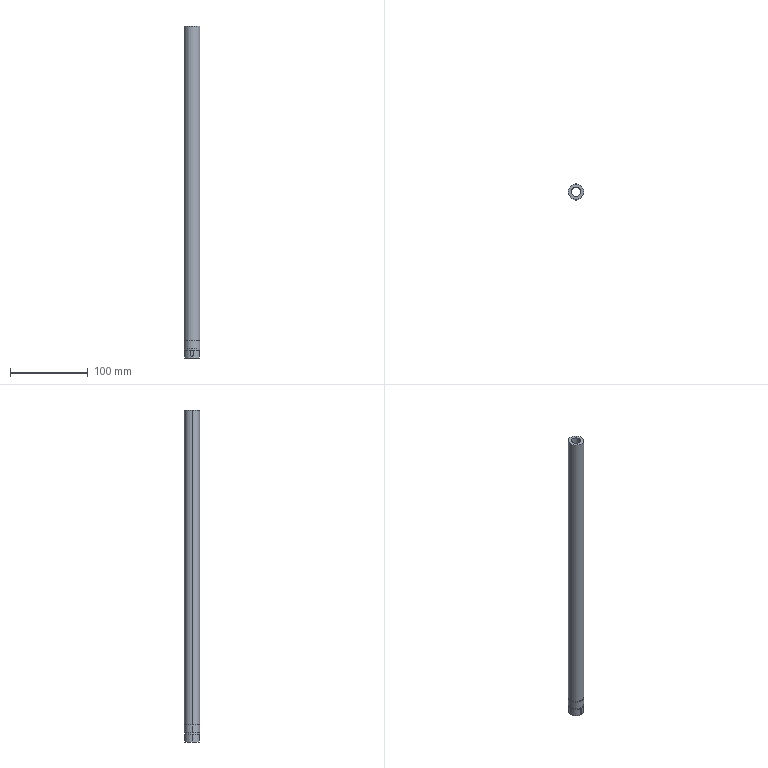Part | SolidWorks | features ICE 11, Extrusion 1 | 1 solid | 33 faces | box 20 x 20 x 428 mm | volume 85566 mm3 | cylinder 18 | plane 15 | commonest cylinder face diameters 3 x6 19 x4 20 x4 12 x2 19.5 x2
STEP:
#1=CARTESIAN_POINT('',(0.,8.2,426.));
#2=VERTEX_POINT('',#1);
#3=CARTESIAN_POINT('',(1.5,8.2,424.5));
#4=VERTEX_POINT('',#3);
#5=CARTESIAN_POINT('',(0.,8.2,424.5));
#6=DIRECTION('',(0.,1.,0.));
#7=DIRECTION('',(0.,0.,1.));
#8=AXIS2_PLACEMENT_3D('',#5,#6,#7);
#9=CIRCLE('',#8,1.5);
#10=EDGE_CURVE('',#2,#4,#9,.T.);
#11=ORIENTED_EDGE('',*,*,#10,.F.);
#12=CARTESIAN_POINT('',(0.,10.,426.));
#13=VERTEX_POINT('',#12);
#14=CARTESIAN_POINT('',(0.,8.2,426.));
#15=DIRECTION('',(0.,1.,0.));
#16=VECTOR('',#15,1000.);
#17=LINE('',#14,#16);
#18=EDGE_CURVE('',#2,#13,#17,.T.);
#19=ORIENTED_EDGE('',*,*,#18,.T.);
#20=CARTESIAN_POINT('',(1.5,9.887,424.5));
#21=VERTEX_POINT('',#20);
#22=CARTESIAN_POINT('',(1.5,9.887,424.5));
#23=CARTESIAN_POINT('',(1.5,9.887,424.599));
#24=CARTESIAN_POINT('',(1.49,9.888,424.697));
#25=CARTESIAN_POINT('',(1.452,9.894,424.889));
#26=CARTESIAN_POINT('',(1.423,9.898,424.984));
#27=CARTESIAN_POINT('',(1.348,9.909,425.166));
#28=CARTESIAN_POINT('',(1.302,9.915,425.252));
#29=CARTESIAN_POINT('',(1.193,9.929,425.415));
#30=CARTESIAN_POINT('',(1.129,9.936,425.492));
#31=CARTESIAN_POINT('',(0.922,9.958,425.699));
#32=CARTESIAN_POINT('',(0.7548,9.973,425.811));
#33=CARTESIAN_POINT('',(0.3937,9.994,425.961));
#34=CARTESIAN_POINT('',(0.196,10.,426.));
#35=CARTESIAN_POINT('',(0.,10.,426.));
#36=B_SPLINE_CURVE_WITH_KNOTS('',3,(#22,#23,#24,#25,#26,#27,#28,#29,#30,#31,#32,#33,#34,#35),.UNSPECIFIED.,.F.,.F.,(4,2,2,2,2,2,4),(0.,0.0002936,0.0005872,0.0008808,0.001174,0.001762,0.002349),.UNSPECIFIED.);
#37=EDGE_CURVE('',#21,#13,#36,.T.);
#38=ORIENTED_EDGE('',*,*,#37,.F.);
#39=CARTESIAN_POINT('',(1.5,8.2,424.5));
#40=DIRECTION('',(0.,1.,0.));
#41=VECTOR('',#40,1000.);
#42=LINE('',#39,#41);
#43=EDGE_CURVE('',#4,#21,#42,.T.);
#44=ORIENTED_EDGE('',*,*,#43,.F.);
#45=EDGE_LOOP('',(#11,#19,#38,#44));
#46=FACE_OUTER_BOUND('',#45,.T.);
#47=CARTESIAN_POINT('',(0.,8.2,424.5));
#48=DIRECTION('',(0.,1.,0.));
#49=DIRECTION('',(0.,0.,1.));
#50=AXIS2_PLACEMENT_3D('',#47,#48,#49);
#51=CYLINDRICAL_SURFACE('',#50,1.5);
#52=ADVANCED_FACE('',(#46),#51,.F.);
#53=CARTESIAN_POINT('',(1.5,9.887,419.5));
#54=VERTEX_POINT('',#53);
#55=CARTESIAN_POINT('',(1.5,9.887,29.));
#56=DIRECTION('',(0.,0.,1.));
#57=VECTOR('',#56,1000.);
#58=LINE('',#55,#57);
#59=EDGE_CURVE('',#54,#21,#58,.T.);
#60=ORIENTED_EDGE('',*,*,#59,.T.);
#61=ORIENTED_EDGE('',*,*,#37,.T.);
#62=CARTESIAN_POINT('',(-1.5,9.887,424.5));
#63=VERTEX_POINT('',#62);
#64=CARTESIAN_POINT('',(0.,10.,426.));
#65=CARTESIAN_POINT('',(-0.09792,10.,426.));
#66=CARTESIAN_POINT('',(-0.1974,9.999,425.99));
#67=CARTESIAN_POINT('',(-0.3897,9.993,425.952));
#68=CARTESIAN_POINT('',(-0.4832,9.989,425.923));
#69=CARTESIAN_POINT('',(-0.7557,9.973,425.811));
#70=CARTESIAN_POINT('',(-0.9207,9.959,425.701));
#71=CARTESIAN_POINT('',(-1.13,9.936,425.491));
#72=CARTESIAN_POINT('',(-1.192,9.929,425.416));
#73=CARTESIAN_POINT('',(-1.301,9.915,425.253));
#74=CARTESIAN_POINT('',(-1.348,9.909,425.166));
#75=CARTESIAN_POINT('',(-1.461,9.893,424.894));
#76=CARTESIAN_POINT('',(-1.5,9.887,424.698));
#77=CARTESIAN_POINT('',(-1.5,9.887,424.5));
#78=B_SPLINE_CURVE_WITH_KNOTS('',3,(#64,#65,#66,#67,#68,#69,#70,#71,#72,#73,#74,#75,#76,#77),.UNSPECIFIED.,.F.,.F.,(4,2,2,2,2,2,4),(0.002349,0.002642,0.002935,0.003522,0.003815,0.004109,0.004695),.UNSPECIFIED.);
#79=EDGE_CURVE('',#13,#63,#78,.T.);
#80=ORIENTED_EDGE('',*,*,#79,.T.);
#81=CARTESIAN_POINT('',(-1.5,9.887,419.5));
#82=VERTEX_POINT('',#81);
#83=CARTESIAN_POINT('',(-1.5,9.887,29.));
#84=DIRECTION('',(0.,0.,-1.));
#85=VECTOR('',#84,1000.);
#86=LINE('',#83,#85);
#87=EDGE_CURVE('',#63,#82,#86,.T.);
#88=ORIENTED_EDGE('',*,*,#87,.T.);
#89=CARTESIAN_POINT('',(-1.5,9.887,419.5));
#90=CARTESIAN_POINT('',(-1.5,9.887,419.401));
#91=CARTESIAN_POINT('',(-1.49,9.888,419.303));
#92=CARTESIAN_POINT('',(-1.452,9.894,419.111));
#93=CARTESIAN_POINT('',(-1.423,9.898,419.016));
#94=CARTESIAN_POINT('',(-1.348,9.909,418.834));
#95=CARTESIAN_POINT('',(-1.302,9.915,418.748));
#96=CARTESIAN_POINT('',(-1.193,9.929,418.585));
#97=CARTESIAN_POINT('',(-1.13,9.936,418.508));
#98=CARTESIAN_POINT('',(-0.9225,9.958,418.301));
#99=CARTESIAN_POINT('',(-0.7554,9.973,418.189));
#100=CARTESIAN_POINT('',(-0.3946,9.994,418.04));
#101=CARTESIAN_POINT('',(-0.1971,10.,418.));
#102=CARTESIAN_POINT('',(0.09684,10.,418.));
#103=CARTESIAN_POINT('',(0.1964,9.999,418.01));
#104=CARTESIAN_POINT('',(0.3888,9.993,418.048));
#105=CARTESIAN_POINT('',(0.4824,9.989,418.076));
#106=CARTESIAN_POINT('',(0.7551,9.973,418.189));
#107=CARTESIAN_POINT('',(0.9202,9.959,418.299));
#108=CARTESIAN_POINT('',(1.13,9.936,418.509));
#109=CARTESIAN_POINT('',(1.192,9.929,418.584));
#110=CARTESIAN_POINT('',(1.301,9.915,418.746));
#111=CARTESIAN_POINT('',(1.348,9.909,418.834));
#112=CARTESIAN_POINT('',(1.461,9.893,419.106));
#113=CARTESIAN_POINT('',(1.5,9.887,419.302));
#114=CARTESIAN_POINT('',(1.5,9.887,419.5));
#115=B_SPLINE_CURVE_WITH_KNOTS('',3,(#89,#90,#91,#92,#93,#94,#95,#96,#97,#98,#99,#100,#101,#102,#103,#104,#105,#106,#107,#108,#109,#110,#111,#112,#113,#114),.UNSPECIFIED.,.F.,.F.,(4,2,2,2,2,2,2,2,2,2,2,2,4),(0.,0.0002934,0.0005869,0.0008803,0.001174,0.001761,0.002348,0.002641,0.002934,0.003521,0.003815,0.004108,0.004695),.UNSPECIFIED.);
#116=EDGE_CURVE('',#82,#54,#115,.T.);
#117=ORIENTED_EDGE('',*,*,#116,.T.);
#118=EDGE_LOOP('',(#60,#61,#80,#88,#117));
#119=FACE_BOUND('',#118,.T.);
#120=CARTESIAN_POINT('',(10.,0.,428.));
#121=VERTEX_POINT('',#120);
#122=CARTESIAN_POINT('',(-10.,0.,428.));
#123=VERTEX_POINT('',#122);
#124=CARTESIAN_POINT('',(0.,0.,428.));
#125=DIRECTION('',(0.,0.,1.));
#126=DIRECTION('',(1.,0.,0.));
#127=AXIS2_PLACEMENT_3D('',#124,#125,#126);
#128=CIRCLE('',#127,10.);
#129=EDGE_CURVE('',#121,#123,#128,.T.);
#130=ORIENTED_EDGE('',*,*,#129,.F.);
#131=CARTESIAN_POINT('',(10.,0.,23.));
#132=VERTEX_POINT('',#131);
#133=CARTESIAN_POINT('',(10.,0.,29.));
#134=DIRECTION('',(0.,0.,-1.));
#135=VECTOR('',#134,1000.);
#136=LINE('',#133,#135);
#137=EDGE_CURVE('',#121,#132,#136,.T.);
#138=ORIENTED_EDGE('',*,*,#137,.T.);
#139=CARTESIAN_POINT('',(-10.,0.,23.));
#140=VERTEX_POINT('',#139);
#141=CARTESIAN_POINT('',(0.,0.,23.));
#142=DIRECTION('',(0.,0.,1.));
#143=DIRECTION('',(1.,0.,0.));
#144=AXIS2_PLACEMENT_3D('',#141,#142,#143);
#145=CIRCLE('',#144,10.);
#146=EDGE_CURVE('',#132,#140,#145,.T.);
#147=ORIENTED_EDGE('',*,*,#146,.T.);
#148=CARTESIAN_POINT('',(-10.,0.,29.));
#149=DIRECTION('',(0.,0.,-1.));
#150=VECTOR('',#149,1000.);
#151=LINE('',#148,#150);
#152=EDGE_CURVE('',#123,#140,#151,.T.);
#153=ORIENTED_EDGE('',*,*,#152,.F.);
#154=EDGE_LOOP('',(#130,#138,#147,#153));
#155=FACE_OUTER_BOUND('',#154,.T.);
#156=CARTESIAN_POINT('',(0.,0.,29.));
#157=DIRECTION('',(0.,0.,-1.));
#158=DIRECTION('',(-1.,0.,0.));
#159=AXIS2_PLACEMENT_3D('',#156,#157,#158);
#160=CYLINDRICAL_SURFACE('',#159,10.);
#161=ADVANCED_FACE('',(#119,#155),#160,.T.);
#162=CARTESIAN_POINT('',(9.5,0.,23.));
#163=VERTEX_POINT('',#162);
#164=CARTESIAN_POINT('',(-9.5,0.,23.));
#165=VERTEX_POINT('',#164);
#166=CARTESIAN_POINT('',(0.,0.,23.));
#167=DIRECTION('',(0.,0.,1.));
#168=DIRECTION('',(1.,0.,0.));
#169=AXIS2_PLACEMENT_3D('',#166,#167,#168);
#170=CIRCLE('',#169,9.5);
#171=EDGE_CURVE('',#163,#165,#170,.T.);
#172=ORIENTED_EDGE('',*,*,#171,.F.);
#173=CARTESIAN_POINT('',(9.5,0.,22.));
#174=VERTEX_POINT('',#173);
#175=CARTESIAN_POINT('',(9.5,0.,23.));
#176=DIRECTION('',(0.,0.,-1.));
#177=VECTOR('',#176,1000.);
#178=LINE('',#175,#177);
#179=EDGE_CURVE('',#163,#174,#178,.T.);
#180=ORIENTED_EDGE('',*,*,#179,.T.);
#181=CARTESIAN_POINT('',(-9.5,0.,22.));
#182=VERTEX_POINT('',#181);
#183=CARTESIAN_POINT('',(0.,0.,22.));
#184=DIRECTION('',(0.,0.,1.));
#185=DIRECTION('',(1.,0.,0.));
#186=AXIS2_PLACEMENT_3D('',#183,#184,#185);
#187=CIRCLE('',#186,9.5);
#188=EDGE_CURVE('',#174,#182,#187,.T.);
#189=ORIENTED_EDGE('',*,*,#188,.T.);
#190=CARTESIAN_POINT('',(-9.5,0.,23.));
#191=DIRECTION('',(0.,0.,-1.));
#192=VECTOR('',#191,1000.);
#193=LINE('',#190,#192);
#194=EDGE_CURVE('',#165,#182,#193,.T.);
#195=ORIENTED_EDGE('',*,*,#194,.F.);
#196=EDGE_LOOP('',(#172,#180,#189,#195));
#197=FACE_OUTER_BOUND('',#196,.T.);
#198=CARTESIAN_POINT('',(0.,0.,23.));
#199=DIRECTION('',(0.,0.,-1.));
#200=DIRECTION('',(-1.,0.,0.));
#201=AXIS2_PLACEMENT_3D('',#198,#199,#200);
#202=CYLINDRICAL_SURFACE('',#201,9.5);
#203=ADVANCED_FACE('',(#197),#202,.T.);
#204=CARTESIAN_POINT('',(10.,0.,22.));
#205=VERTEX_POINT('',#204);
#206=CARTESIAN_POINT('',(-10.,0.,22.));
#207=VERTEX_POINT('',#206);
#208=CARTESIAN_POINT('',(0.,0.,22.));
#209=DIRECTION('',(0.,0.,1.));
#210=DIRECTION('',(1.,0.,0.));
#211=AXIS2_PLACEMENT_3D('',#208,#209,#210);
#212=CIRCLE('',#211,10.);
#213=EDGE_CURVE('',#205,#207,#212,.T.);
#214=ORIENTED_EDGE('',*,*,#213,.F.);
#215=CARTESIAN_POINT('',(10.,0.,12.));
#216=VERTEX_POINT('',#215);
#217=CARTESIAN_POINT('',(10.,0.,22.));
#218=DIRECTION('',(0.,0.,-1.));
#219=VECTOR('',#218,1000.);
#220=LINE('',#217,#219);
#221=EDGE_CURVE('',#205,#216,#220,.T.);
#222=ORIENTED_EDGE('',*,*,#221,.T.);
#223=CARTESIAN_POINT('',(-10.,0.,12.));
#224=VERTEX_POINT('',#223);
#225=CARTESIAN_POINT('',(0.,0.,12.));
#226=DIRECTION('',(0.,0.,1.));
#227=DIRECTION('',(1.,0.,0.));
#228=AXIS2_PLACEMENT_3D('',#225,#226,#227);
#229=CIRCLE('',#228,10.);
#230=EDGE_CURVE('',#216,#224,#229,.T.);
#231=ORIENTED_EDGE('',*,*,#230,.T.);
#232=CARTESIAN_POINT('',(-10.,0.,22.));
#233=DIRECTION('',(0.,0.,-1.));
#234=VECTOR('',#233,1000.);
#235=LINE('',#232,#234);
#236=EDGE_CURVE('',#207,#224,#235,.T.);
#237=ORIENTED_EDGE('',*,*,#236,.F.);
#238=EDGE_LOOP('',(#214,#222,#231,#237));
#239=FACE_OUTER_BOUND('',#238,.T.);
#240=CARTESIAN_POINT('',(0.,0.,22.));
#241=DIRECTION('',(0.,0.,-1.));
#242=DIRECTION('',(-1.,0.,0.));
#243=AXIS2_PLACEMENT_3D('',#240,#241,#242);
#244=CYLINDRICAL_SURFACE('',#243,10.);
#245=ADVANCED_FACE('',(#239),#244,.T.);
#246=CARTESIAN_POINT('',(9.75,0.,12.));
#247=VERTEX_POINT('',#246);
#248=CARTESIAN_POINT('',(-9.75,0.,12.));
#249=VERTEX_POINT('',#248);
#250=CARTESIAN_POINT('',(0.,0.,12.));
#251=DIRECTION('',(0.,0.,1.));
#252=DIRECTION('',(1.,0.,0.));
#253=AXIS2_PLACEMENT_3D('',#250,#251,#252);
#254=CIRCLE('',#253,9.75);
#255=EDGE_CURVE('',#247,#249,#254,.T.);
#256=ORIENTED_EDGE('',*,*,#255,.F.);
#257=CARTESIAN_POINT('',(9.75,0.,10.));
#258=VERTEX_POINT('',#257);
#259=CARTESIAN_POINT('',(9.75,0.,12.));
#260=DIRECTION('',(0.,0.,-1.));
#261=VECTOR('',#260,1000.);
#262=LINE('',#259,#261);
#263=EDGE_CURVE('',#247,#258,#262,.T.);
#264=ORIENTED_EDGE('',*,*,#263,.T.);
#265=CARTESIAN_POINT('',(-9.75,0.,10.));
#266=VERTEX_POINT('',#265);
#267=CARTESIAN_POINT('',(0.,0.,10.));
#268=DIRECTION('',(0.,0.,1.));
#269=DIRECTION('',(1.,0.,0.));
#270=AXIS2_PLACEMENT_3D('',#267,#268,#269);
#271=CIRCLE('',#270,9.75);
#272=EDGE_CURVE('',#258,#266,#271,.T.);
#273=ORIENTED_EDGE('',*,*,#272,.T.);
#274=CARTESIAN_POINT('',(-9.75,0.,12.));
#275=DIRECTION('',(0.,0.,-1.));
#276=VECTOR('',#275,1000.);
#277=LINE('',#274,#276);
#278=EDGE_CURVE('',#249,#266,#277,.T.);
#279=ORIENTED_EDGE('',*,*,#278,.F.);
#280=EDGE_LOOP('',(#256,#264,#273,#279));
#281=FACE_OUTER_BOUND('',#280,.T.);
#282=CARTESIAN_POINT('',(0.,0.,12.));
#283=DIRECTION('',(0.,0.,-1.));
#284=DIRECTION('',(-1.,0.,0.));
#285=AXIS2_PLACEMENT_3D('',#282,#283,#284);
#286=CYLINDRICAL_SURFACE('',#285,9.75);
#287=ADVANCED_FACE('',(#281),#286,.T.);
#288=CARTESIAN_POINT('',(1.5,-7.7,3.5));
#289=VERTEX_POINT('',#288);
#290=CARTESIAN_POINT('',(0.,-7.7,2.));
#291=VERTEX_POINT('',#290);
#292=CARTESIAN_POINT('',(0.,-7.7,3.5));
#293=DIRECTION('',(0.,1.,0.));
#294=DIRECTION('',(0.,0.,1.));
#295=AXIS2_PLACEMENT_3D('',#292,#293,#294);
#296=CIRCLE('',#295,1.5);
#297=EDGE_CURVE('',#289,#291,#296,.T.);
#298=ORIENTED_EDGE('',*,*,#297,.T.);
#299=CARTESIAN_POINT('',(0.,-9.5,2.));
#300=VERTEX_POINT('',#299);
#301=CARTESIAN_POINT('',(0.,-7.7,2.));
#302=DIRECTION('',(0.,-1.,0.));
#303=VECTOR('',#302,1000.);
#304=LINE('',#301,#303);
#305=EDGE_CURVE('',#291,#300,#304,.T.);
#306=ORIENTED_EDGE('',*,*,#305,.T.);
#307=CARTESIAN_POINT('',(1.5,-9.381,3.5));
#308=VERTEX_POINT('',#307);
#309=CARTESIAN_POINT('',(0.,-9.5,2.));
#310=CARTESIAN_POINT('',(0.09794,-9.5,2.));
#311=CARTESIAN_POINT('',(0.1974,-9.498,2.01));
#312=CARTESIAN_POINT('',(0.3898,-9.492,2.048));
#313=CARTESIAN_POINT('',(0.4833,-9.488,2.077));
#314=CARTESIAN_POINT('',(0.7558,-9.472,2.189));
#315=CARTESIAN_POINT('',(0.9208,-9.456,2.299));
#316=CARTESIAN_POINT('',(1.13,-9.433,2.509));
#317=CARTESIAN_POINT('',(1.192,-9.425,2.584));
#318=CARTESIAN_POINT('',(1.301,-9.411,2.747));
#319=CARTESIAN_POINT('',(1.348,-9.404,2.834));
#320=CARTESIAN_POINT('',(1.461,-9.387,3.106));
#321=CARTESIAN_POINT('',(1.5,-9.381,3.302));
#322=CARTESIAN_POINT('',(1.5,-9.381,3.5));
#323=B_SPLINE_CURVE_WITH_KNOTS('',3,(#309,#310,#311,#312,#313,#314,#315,#316,#317,#318,#319,#320,#321,#322),.UNSPECIFIED.,.F.,.F.,(4,2,2,2,2,2,4),(0.002349,0.002642,0.002936,0.003522,0.003816,0.004109,0.004696),.UNSPECIFIED.);
#324=EDGE_CURVE('',#300,#308,#323,.T.);
#325=ORIENTED_EDGE('',*,*,#324,.T.);
#326=CARTESIAN_POINT('',(1.5,-7.7,3.5));
#327=DIRECTION('',(0.,-1.,0.));
#328=VECTOR('',#327,1000.);
#329=LINE('',#326,#328);
#330=EDGE_CURVE('',#289,#308,#329,.T.);
#331=ORIENTED_EDGE('',*,*,#330,.F.);
#332=EDGE_LOOP('',(#298,#306,#325,#331));
#333=FACE_OUTER_BOUND('',#332,.T.);
#334=CARTESIAN_POINT('',(0.,-7.7,3.5));
#335=DIRECTION('',(0.,-1.,0.));
#336=DIRECTION('',(0.,0.,-1.));
#337=AXIS2_PLACEMENT_3D('',#334,#335,#336);
#338=CYLINDRICAL_SURFACE('',#337,1.5);
#339=ADVANCED_FACE('',(#333),#338,.F.);
#340=CARTESIAN_POINT('',(-6.,0.,428.));
#341=VERTEX_POINT('',#340);
#342=CARTESIAN_POINT('',(6.,0.,428.));
#343=VERTEX_POINT('',#342);
#344=CARTESIAN_POINT('',(0.,0.,428.));
#345=DIRECTION('',(0.,0.,1.));
#346=DIRECTION('',(1.,0.,0.));
#347=AXIS2_PLACEMENT_3D('',#344,#345,#346);
#348=CIRCLE('',#347,6.);
#349=EDGE_CURVE('',#341,#343,#348,.T.);
#350=ORIENTED_EDGE('',*,*,#349,.T.);
#351=CARTESIAN_POINT('',(6.,0.,0.));
#352=VERTEX_POINT('',#351);
#353=CARTESIAN_POINT('',(6.,0.,10.));
#354=DIRECTION('',(0.,0.,-1.));
#355=VECTOR('',#354,1000.);
#356=LINE('',#353,#355);
#357=EDGE_CURVE('',#343,#352,#356,.T.);
#358=ORIENTED_EDGE('',*,*,#357,.T.);
#359=CARTESIAN_POINT('',(-6.,0.,0.));
#360=VERTEX_POINT('',#359);
#361=CARTESIAN_POINT('',(0.,0.,0.));
#362=DIRECTION('',(0.,0.,1.));
#363=DIRECTION('',(1.,0.,0.));
#364=AXIS2_PLACEMENT_3D('',#361,#362,#363);
#365=CIRCLE('',#364,6.);
#366=EDGE_CURVE('',#360,#352,#365,.T.);
#367=ORIENTED_EDGE('',*,*,#366,.F.);
#368=CARTESIAN_POINT('',(-6.,0.,10.));
#369=DIRECTION('',(0.,0.,-1.));
#370=VECTOR('',#369,1000.);
#371=LINE('',#368,#370);
#372=EDGE_CURVE('',#341,#360,#371,.T.);
#373=ORIENTED_EDGE('',*,*,#372,.F.);
#374=EDGE_LOOP('',(#350,#358,#367,#373));
#375=FACE_OUTER_BOUND('',#374,.T.);
#376=CARTESIAN_POINT('',(0.,0.,10.));
#377=DIRECTION('',(0.,0.,-1.));
#378=DIRECTION('',(-1.,0.,0.));
#379=AXIS2_PLACEMENT_3D('',#376,#377,#378);
#380=CYLINDRICAL_SURFACE('',#379,6.);
#381=ADVANCED_FACE('',(#375),#380,.F.);
#382=CARTESIAN_POINT('',(9.5,0.,10.));
#383=VERTEX_POINT('',#382);
#384=CARTESIAN_POINT('',(1.5,9.381,10.));
#385=VERTEX_POINT('',#384);
#386=CARTESIAN_POINT('',(0.,0.,10.));
#387=DIRECTION('',(0.,0.,1.));
#388=DIRECTION('',(1.,0.,0.));
#389=AXIS2_PLACEMENT_3D('',#386,#387,#388);
#390=CIRCLE('',#389,9.5);
#391=EDGE_CURVE('',#383,#385,#390,.T.);
#392=ORIENTED_EDGE('',*,*,#391,.F.);
#393=CARTESIAN_POINT('',(9.5,0.,0.));
#394=VERTEX_POINT('',#393);
#395=CARTESIAN_POINT('',(9.5,0.,10.));
#396=DIRECTION('',(0.,0.,-1.));
#397=VECTOR('',#396,1000.);
#398=LINE('',#395,#397);
#399=EDGE_CURVE('',#383,#394,#398,.T.);
#400=ORIENTED_EDGE('',*,*,#399,.T.);
#401=CARTESIAN_POINT('',(-9.5,0.,0.));
#402=VERTEX_POINT('',#401);
#403=CARTESIAN_POINT('',(0.,0.,0.));
#404=DIRECTION('',(0.,0.,1.));
#405=DIRECTION('',(1.,0.,0.));
#406=AXIS2_PLACEMENT_3D('',#403,#404,#405);
#407=CIRCLE('',#406,9.5);
#408=EDGE_CURVE('',#394,#402,#407,.T.);
#409=ORIENTED_EDGE('',*,*,#408,.T.);
#410=CARTESIAN_POINT('',(-9.5,0.,10.));
#411=VERTEX_POINT('',#410);
#412=CARTESIAN_POINT('',(-9.5,0.,10.));
#413=DIRECTION('',(0.,0.,-1.));
#414=VECTOR('',#413,1000.);
#415=LINE('',#412,#414);
#416=EDGE_CURVE('',#411,#402,#415,.T.);
#417=ORIENTED_EDGE('',*,*,#416,.F.);
#418=CARTESIAN_POINT('',(-1.5,9.381,10.));
#419=VERTEX_POINT('',#418);
#420=CARTESIAN_POINT('',(0.,0.,10.));
#421=DIRECTION('',(0.,0.,1.));
#422=DIRECTION('',(1.,0.,0.));
#423=AXIS2_PLACEMENT_3D('',#420,#421,#422);
#424=CIRCLE('',#423,9.5);
#425=EDGE_CURVE('',#419,#411,#424,.T.);
#426=ORIENTED_EDGE('',*,*,#425,.F.);
#427=CARTESIAN_POINT('',(-1.5,9.381,3.5));
#428=VERTEX_POINT('',#427);
#429=CARTESIAN_POINT('',(-1.5,9.381,10.));
#430=DIRECTION('',(0.,0.,-1.));
#431=VECTOR('',#430,1000.);
#432=LINE('',#429,#431);
#433=EDGE_CURVE('',#419,#428,#432,.T.);
#434=ORIENTED_EDGE('',*,*,#433,.T.);
#435=CARTESIAN_POINT('',(1.5,9.381,3.5));
#436=VERTEX_POINT('',#435);
#437=CARTESIAN_POINT('',(-1.5,9.381,3.5));
#438=CARTESIAN_POINT('',(-1.5,9.381,3.401));
#439=CARTESIAN_POINT('',(-1.49,9.382,3.303));
#440=CARTESIAN_POINT('',(-1.452,9.388,3.111));
#441=CARTESIAN_POINT('',(-1.423,9.393,3.016));
#442=CARTESIAN_POINT('',(-1.348,9.404,2.834));
#443=CARTESIAN_POINT('',(-1.302,9.411,2.748));
#444=CARTESIAN_POINT('',(-1.193,9.425,2.585));
#445=CARTESIAN_POINT('',(-1.13,9.433,2.508));
#446=CARTESIAN_POINT('',(-0.9225,9.456,2.301));
#447=CARTESIAN_POINT('',(-0.7555,9.472,2.189));
#448=CARTESIAN_POINT('',(-0.3947,9.494,2.04));
#449=CARTESIAN_POINT('',(-0.1971,9.5,2.));
#450=CARTESIAN_POINT('',(0.09684,9.5,2.));
#451=CARTESIAN_POINT('',(0.1964,9.498,2.01));
#452=CARTESIAN_POINT('',(0.3889,9.493,2.048));
#453=CARTESIAN_POINT('',(0.4824,9.488,2.076));
#454=CARTESIAN_POINT('',(0.7551,9.472,2.189));
#455=CARTESIAN_POINT('',(0.9202,9.456,2.299));
#456=CARTESIAN_POINT('',(1.13,9.433,2.509));
#457=CARTESIAN_POINT('',(1.192,9.425,2.584));
#458=CARTESIAN_POINT('',(1.301,9.411,2.746));
#459=CARTESIAN_POINT('',(1.348,9.404,2.834));
#460=CARTESIAN_POINT('',(1.461,9.387,3.106));
#461=CARTESIAN_POINT('',(1.5,9.381,3.301));
#462=CARTESIAN_POINT('',(1.5,9.381,3.5));
#463=B_SPLINE_CURVE_WITH_KNOTS('',3,(#437,#438,#439,#440,#441,#442,#443,#444,#445,#446,#447,#448,#449,#450,#451,#452,#453,#454,#455,#456,#457,#458,#459,#460,#461,#462),.UNSPECIFIED.,.F.,.F.,(4,2,2,2,2,2,2,2,2,2,2,2,4),(0.,0.0002935,0.000587,0.0008805,0.001174,0.001761,0.002348,0.002641,0.002935,0.003522,0.003815,0.004109,0.004696),.UNSPECIFIED.);
#464=EDGE_CURVE('',#428,#436,#463,.T.);
#465=ORIENTED_EDGE('',*,*,#464,.T.);
#466=CARTESIAN_POINT('',(1.5,9.381,10.));
#467=DIRECTION('',(0.,0.,1.));
#468=VECTOR('',#467,1000.);
#469=LINE('',#466,#468);
#470=EDGE_CURVE('',#436,#385,#469,.T.);
#471=ORIENTED_EDGE('',*,*,#470,.T.);
#472=EDGE_LOOP('',(#392,#400,#409,#417,#426,#434,#465,#471));
#473=FACE_OUTER_BOUND('',#472,.T.);
#474=CARTESIAN_POINT('',(0.,0.,10.));
#475=DIRECTION('',(0.,0.,-1.));
#476=DIRECTION('',(-1.,0.,0.));
#477=AXIS2_PLACEMENT_3D('',#474,#475,#476);
#478=CYLINDRICAL_SURFACE('',#477,9.5);
#479=ADVANCED_FACE('',(#473),#478,.T.);
#480=ORIENTED_EDGE('',*,*,#399,.F.);
#481=CARTESIAN_POINT('',(1.5,-9.381,10.));
#482=VERTEX_POINT('',#481);
#483=CARTESIAN_POINT('',(0.,0.,10.));
#484=DIRECTION('',(0.,0.,1.));
#485=DIRECTION('',(1.,0.,0.));
#486=AXIS2_PLACEMENT_3D('',#483,#484,#485);
#487=CIRCLE('',#486,9.5);
#488=EDGE_CURVE('',#482,#383,#487,.T.);
#489=ORIENTED_EDGE('',*,*,#488,.F.);
#490=CARTESIAN_POINT('',(1.5,-9.381,10.));
#491=DIRECTION('',(0.,0.,1.));
#492=VECTOR('',#491,1000.);
#493=LINE('',#490,#492);
#494=EDGE_CURVE('',#308,#482,#493,.T.);
#495=ORIENTED_EDGE('',*,*,#494,.F.);
#496=ORIENTED_EDGE('',*,*,#324,.F.);
#497=CARTESIAN_POINT('',(-1.5,-9.381,3.5));
#498=VERTEX_POINT('',#497);
#499=CARTESIAN_POINT('',(-1.5,-9.381,3.5));
#500=CARTESIAN_POINT('',(-1.5,-9.381,3.401));
#501=CARTESIAN_POINT('',(-1.49,-9.382,3.303));
#502=CARTESIAN_POINT('',(-1.452,-9.388,3.111));
#503=CARTESIAN_POINT('',(-1.423,-9.393,3.016));
#504=CARTESIAN_POINT('',(-1.348,-9.404,2.834));
#505=CARTESIAN_POINT('',(-1.302,-9.411,2.748));
#506=CARTESIAN_POINT('',(-1.193,-9.425,2.585));
#507=CARTESIAN_POINT('',(-1.129,-9.433,2.508));
#508=CARTESIAN_POINT('',(-0.922,-9.456,2.301));
#509=CARTESIAN_POINT('',(-0.7548,-9.472,2.189));
#510=CARTESIAN_POINT('',(-0.3938,-9.494,2.039));
#511=CARTESIAN_POINT('',(-0.1961,-9.5,2.));
#512=CARTESIAN_POINT('',(0.,-9.5,2.));
#513=B_SPLINE_CURVE_WITH_KNOTS('',3,(#499,#500,#501,#502,#503,#504,#505,#506,#507,#508,#509,#510,#511,#512),.UNSPECIFIED.,.F.,.F.,(4,2,2,2,2,2,4),(0.,0.0002936,0.0005873,0.0008809,0.001175,0.001762,0.002349),.UNSPECIFIED.);
#514=EDGE_CURVE('',#498,#300,#513,.T.);
#515=ORIENTED_EDGE('',*,*,#514,.F.);
#516=CARTESIAN_POINT('',(-1.5,-9.381,10.));
#517=VERTEX_POINT('',#516);
#518=CARTESIAN_POINT('',(-1.5,-9.381,10.));
#519=DIRECTION('',(0.,0.,-1.));
#520=VECTOR('',#519,1000.);
#521=LINE('',#518,#520);
#522=EDGE_CURVE('',#517,#498,#521,.T.);
#523=ORIENTED_EDGE('',*,*,#522,.F.);
#524=CARTESIAN_POINT('',(0.,0.,10.));
#525=DIRECTION('',(0.,0.,1.));
#526=DIRECTION('',(1.,0.,0.));
#527=AXIS2_PLACEMENT_3D('',#524,#525,#526);
#528=CIRCLE('',#527,9.5);
#529=EDGE_CURVE('',#411,#517,#528,.T.);
#530=ORIENTED_EDGE('',*,*,#529,.F.);
#531=ORIENTED_EDGE('',*,*,#416,.T.);
#532=CARTESIAN_POINT('',(0.,0.,0.));
#533=DIRECTION('',(0.,0.,1.));
#534=DIRECTION('',(1.,0.,0.));
#535=AXIS2_PLACEMENT_3D('',#532,#533,#534);
#536=CIRCLE('',#535,9.5);
#537=EDGE_CURVE('',#402,#394,#536,.T.);
#538=ORIENTED_EDGE('',*,*,#537,.T.);
#539=EDGE_LOOP('',(#480,#489,#495,#496,#515,#523,#530,#531,#538));
#540=FACE_OUTER_BOUND('',#539,.T.);
#541=CARTESIAN_POINT('',(0.,0.,10.));
#542=DIRECTION('',(0.,0.,-1.));
#543=DIRECTION('',(-1.,0.,0.));
#544=AXIS2_PLACEMENT_3D('',#541,#542,#543);
#545=CYLINDRICAL_SURFACE('',#544,9.5);
#546=ADVANCED_FACE('',(#540),#545,.T.);
#547=ORIENTED_EDGE('',*,*,#537,.F.);
#548=ORIENTED_EDGE('',*,*,#408,.F.);
#549=EDGE_LOOP('',(#547,#548));
#550=FACE_OUTER_BOUND('',#549,.T.);
#551=ORIENTED_EDGE('',*,*,#366,.T.);
#552=CARTESIAN_POINT('',(0.,0.,0.));
#553=DIRECTION('',(0.,0.,1.));
#554=DIRECTION('',(1.,0.,0.));
#555=AXIS2_PLACEMENT_3D('',#552,#553,#554);
#556=CIRCLE('',#555,6.);
#557=EDGE_CURVE('',#352,#360,#556,.T.);
#558=ORIENTED_EDGE('',*,*,#557,.T.);
#559=EDGE_LOOP('',(#551,#558));
#560=FACE_BOUND('',#559,.T.);
#561=CARTESIAN_POINT('',(0.,0.,0.));
#562=DIRECTION('',(0.,0.,1.));
#563=DIRECTION('',(1.,0.,0.));
#564=AXIS2_PLACEMENT_3D('',#561,#562,#563);
#565=PLANE('',#564);
#566=ADVANCED_FACE('',(#550,#560),#565,.F.);
#567=ORIENTED_EDGE('',*,*,#357,.F.);
#568=CARTESIAN_POINT('',(0.,0.,428.));
#569=DIRECTION('',(0.,0.,1.));
#570=DIRECTION('',(1.,0.,0.));
#571=AXIS2_PLACEMENT_3D('',#568,#569,#570);
#572=CIRCLE('',#571,6.);
#573=EDGE_CURVE('',#343,#341,#572,.T.);
#574=ORIENTED_EDGE('',*,*,#573,.T.);
#575=ORIENTED_EDGE('',*,*,#372,.T.);
#576=ORIENTED_EDGE('',*,*,#557,.F.);
#577=EDGE_LOOP('',(#567,#574,#575,#576));
#578=FACE_OUTER_BOUND('',#577,.T.);
#579=CARTESIAN_POINT('',(0.,0.,10.));
#580=DIRECTION('',(0.,0.,-1.));
#581=DIRECTION('',(-1.,0.,0.));
#582=AXIS2_PLACEMENT_3D('',#579,#580,#581);
#583=CYLINDRICAL_SURFACE('',#582,6.);
#584=ADVANCED_FACE('',(#578),#583,.F.);
#585=CARTESIAN_POINT('',(-1.5,7.7,3.5));
#586=VERTEX_POINT('',#585);
#587=CARTESIAN_POINT('',(-1.5,7.7,3.5));
#588=DIRECTION('',(0.,1.,0.));
#589=VECTOR('',#588,1000.);
#590=LINE('',#587,#589);
#591=EDGE_CURVE('',#586,#428,#590,.T.);
#592=ORIENTED_EDGE('',*,*,#591,.F.);
#593=CARTESIAN_POINT('',(1.5,7.7,3.5));
#594=VERTEX_POINT('',#593);
#595=CARTESIAN_POINT('',(0.,7.7,3.5));
#596=DIRECTION('',(0.,1.,0.));
#597=DIRECTION('',(0.,0.,1.));
#598=AXIS2_PLACEMENT_3D('',#595,#596,#597);
#599=CIRCLE('',#598,1.5);
#600=EDGE_CURVE('',#594,#586,#599,.T.);
#601=ORIENTED_EDGE('',*,*,#600,.F.);
#602=CARTESIAN_POINT('',(1.5,7.7,3.5));
#603=DIRECTION('',(0.,1.,0.));
#604=VECTOR('',#603,1000.);
#605=LINE('',#602,#604);
#606=EDGE_CURVE('',#594,#436,#605,.T.);
#607=ORIENTED_EDGE('',*,*,#606,.T.);
#608=ORIENTED_EDGE('',*,*,#464,.F.);
#609=EDGE_LOOP('',(#592,#601,#607,#608));
#610=FACE_OUTER_BOUND('',#609,.T.);
#611=CARTESIAN_POINT('',(0.,7.7,3.5));
#612=DIRECTION('',(0.,1.,0.));
#613=DIRECTION('',(0.,0.,1.));
#614=AXIS2_PLACEMENT_3D('',#611,#612,#613);
#615=CYLINDRICAL_SURFACE('',#614,1.5);
#616=ADVANCED_FACE('',(#610),#615,.F.);
#617=ORIENTED_EDGE('',*,*,#606,.F.);
#618=CARTESIAN_POINT('',(1.5,7.7,10.));
#619=VERTEX_POINT('',#618);
#620=CARTESIAN_POINT('',(1.5,7.7,10.));
#621=DIRECTION('',(0.,0.,-1.));
#622=VECTOR('',#621,1000.);
#623=LINE('',#620,#622);
#624=EDGE_CURVE('',#619,#594,#623,.T.);
#625=ORIENTED_EDGE('',*,*,#624,.F.);
#626=CARTESIAN_POINT('',(1.5,7.7,10.));
#627=DIRECTION('',(0.,1.,0.));
#628=VECTOR('',#627,1000.);
#629=LINE('',#626,#628);
#630=EDGE_CURVE('',#619,#385,#629,.T.);
#631=ORIENTED_EDGE('',*,*,#630,.T.);
#632=ORIENTED_EDGE('',*,*,#470,.F.);
#633=EDGE_LOOP('',(#617,#625,#631,#632));
#634=FACE_OUTER_BOUND('',#633,.T.);
#635=CARTESIAN_POINT('',(1.5,7.7,3.5));
#636=DIRECTION('',(1.,0.,0.));
#637=DIRECTION('',(0.,0.,-1.));
#638=AXIS2_PLACEMENT_3D('',#635,#636,#637);
#639=PLANE('',#638);
#640=ADVANCED_FACE('',(#634),#639,.F.);
#641=CARTESIAN_POINT('',(-1.5,7.7,10.));
#642=VERTEX_POINT('',#641);
#643=CARTESIAN_POINT('',(-1.5,7.7,10.));
#644=DIRECTION('',(0.,1.,0.));
#645=VECTOR('',#644,1000.);
#646=LINE('',#643,#645);
#647=EDGE_CURVE('',#642,#419,#646,.T.);
#648=ORIENTED_EDGE('',*,*,#647,.F.);
#649=CARTESIAN_POINT('',(-1.5,7.7,3.5));
#650=DIRECTION('',(0.,0.,1.));
#651=VECTOR('',#650,1000.);
#652=LINE('',#649,#651);
#653=EDGE_CURVE('',#586,#642,#652,.T.);
#654=ORIENTED_EDGE('',*,*,#653,.F.);
#655=ORIENTED_EDGE('',*,*,#591,.T.);
#656=ORIENTED_EDGE('',*,*,#433,.F.);
#657=EDGE_LOOP('',(#648,#654,#655,#656));
#658=FACE_OUTER_BOUND('',#657,.T.);
#659=CARTESIAN_POINT('',(-1.5,7.7,8.5));
#660=DIRECTION('',(-1.,0.,0.));
#661=DIRECTION('',(0.,0.,1.));
#662=AXIS2_PLACEMENT_3D('',#659,#660,#661);
#663=PLANE('',#662);
#664=ADVANCED_FACE('',(#658),#663,.F.);
#665=ORIENTED_EDGE('',*,*,#600,.T.);
#666=ORIENTED_EDGE('',*,*,#653,.T.);
#667=CARTESIAN_POINT('',(-1.5,7.7,10.));
#668=DIRECTION('',(1.,0.,0.));
#669=VECTOR('',#668,1000.);
#670=LINE('',#667,#669);
#671=EDGE_CURVE('',#642,#619,#670,.T.);
#672=ORIENTED_EDGE('',*,*,#671,.T.);
#673=ORIENTED_EDGE('',*,*,#624,.T.);
#674=EDGE_LOOP('',(#665,#666,#672,#673));
#675=FACE_OUTER_BOUND('',#674,.T.);
#676=CARTESIAN_POINT('',(0.,7.7,3.5));
#677=DIRECTION('',(0.,1.,0.));
#678=DIRECTION('',(0.,0.,1.));
#679=AXIS2_PLACEMENT_3D('',#676,#677,#678);
#680=PLANE('',#679);
#681=ADVANCED_FACE('',(#675),#680,.T.);
#682=ORIENTED_EDGE('',*,*,#305,.F.);
#683=CARTESIAN_POINT('',(-1.5,-7.7,3.5));
#684=VERTEX_POINT('',#683);
#685=CARTESIAN_POINT('',(0.,-7.7,3.5));
#686=DIRECTION('',(0.,1.,0.));
#687=DIRECTION('',(0.,0.,1.));
#688=AXIS2_PLACEMENT_3D('',#685,#686,#687);
#689=CIRCLE('',#688,1.5);
#690=EDGE_CURVE('',#291,#684,#689,.T.);
#691=ORIENTED_EDGE('',*,*,#690,.T.);
#692=CARTESIAN_POINT('',(-1.5,-7.7,3.5));
#693=DIRECTION('',(0.,-1.,0.));
#694=VECTOR('',#693,1000.);
#695=LINE('',#692,#694);
#696=EDGE_CURVE('',#684,#498,#695,.T.);
#697=ORIENTED_EDGE('',*,*,#696,.T.);
#698=ORIENTED_EDGE('',*,*,#514,.T.);
#699=EDGE_LOOP('',(#682,#691,#697,#698));
#700=FACE_OUTER_BOUND('',#699,.T.);
#701=CARTESIAN_POINT('',(0.,-7.7,3.5));
#702=DIRECTION('',(0.,-1.,0.));
#703=DIRECTION('',(0.,0.,-1.));
#704=AXIS2_PLACEMENT_3D('',#701,#702,#703);
#705=CYLINDRICAL_SURFACE('',#704,1.5);
#706=ADVANCED_FACE('',(#700),#705,.F.);
#707=ORIENTED_EDGE('',*,*,#522,.T.);
#708=ORIENTED_EDGE('',*,*,#696,.F.);
#709=CARTESIAN_POINT('',(-1.5,-7.7,10.));
#710=VERTEX_POINT('',#709);
#711=CARTESIAN_POINT('',(-1.5,-7.7,3.5));
#712=DIRECTION('',(0.,0.,1.));
#713=VECTOR('',#712,1000.);
#714=LINE('',#711,#713);
#715=EDGE_CURVE('',#684,#710,#714,.T.);
#716=ORIENTED_EDGE('',*,*,#715,.T.);
#717=CARTESIAN_POINT('',(-1.5,0.,10.));
#718=DIRECTION('',(0.,1.,0.));
#719=VECTOR('',#718,1000.);
#720=LINE('',#717,#719);
#721=EDGE_CURVE('',#517,#710,#720,.T.);
#722=ORIENTED_EDGE('',*,*,#721,.F.);
#723=EDGE_LOOP('',(#707,#708,#716,#722));
#724=FACE_OUTER_BOUND('',#723,.T.);
#725=CARTESIAN_POINT('',(-1.5,-7.7,10.031));
#726=DIRECTION('',(1.,0.,0.));
#727=DIRECTION('',(0.,0.,-1.));
#728=AXIS2_PLACEMENT_3D('',#725,#726,#727);
#729=PLANE('',#728);
#730=ADVANCED_FACE('',(#724),#729,.T.);
#731=CARTESIAN_POINT('',(1.5,-7.7,10.));
#732=VERTEX_POINT('',#731);
#733=CARTESIAN_POINT('',(1.5,-7.7,8.5));
#734=DIRECTION('',(0.,0.,-1.));
#735=VECTOR('',#734,1000.);
#736=LINE('',#733,#735);
#737=EDGE_CURVE('',#732,#289,#736,.T.);
#738=ORIENTED_EDGE('',*,*,#737,.T.);
#739=ORIENTED_EDGE('',*,*,#330,.T.);
#740=ORIENTED_EDGE('',*,*,#494,.T.);
#741=CARTESIAN_POINT('',(1.5,0.,10.));
#742=DIRECTION('',(0.,-1.,0.));
#743=VECTOR('',#742,1000.);
#744=LINE('',#741,#743);
#745=EDGE_CURVE('',#732,#482,#744,.T.);
#746=ORIENTED_EDGE('',*,*,#745,.F.);
#747=EDGE_LOOP('',(#738,#739,#740,#746));
#748=FACE_OUTER_BOUND('',#747,.T.);
#749=CARTESIAN_POINT('',(1.5,-7.7,3.5));
#750=DIRECTION('',(-1.,0.,0.));
#751=DIRECTION('',(0.,0.,1.));
#752=AXIS2_PLACEMENT_3D('',#749,#750,#751);
#753=PLANE('',#752);
#754=ADVANCED_FACE('',(#748),#753,.T.);
#755=CARTESIAN_POINT('',(0.,-7.7,10.));
#756=DIRECTION('',(-1.,0.,0.));
#757=VECTOR('',#756,1000.);
#758=LINE('',#755,#757);
#759=EDGE_CURVE('',#732,#710,#758,.T.);
#760=ORIENTED_EDGE('',*,*,#759,.T.);
#761=ORIENTED_EDGE('',*,*,#715,.F.);
#762=ORIENTED_EDGE('',*,*,#690,.F.);
#763=ORIENTED_EDGE('',*,*,#297,.F.);
#764=ORIENTED_EDGE('',*,*,#737,.F.);
#765=EDGE_LOOP('',(#760,#761,#762,#763,#764));
#766=FACE_OUTER_BOUND('',#765,.T.);
#767=CARTESIAN_POINT('',(0.,-7.7,3.5));
#768=DIRECTION('',(0.,1.,0.));
#769=DIRECTION('',(0.,0.,1.));
#770=AXIS2_PLACEMENT_3D('',#767,#768,#769);
#771=PLANE('',#770);
#772=ADVANCED_FACE('',(#766),#771,.F.);
#773=CARTESIAN_POINT('',(0.,0.,10.));
#774=DIRECTION('',(0.,0.,1.));
#775=DIRECTION('',(1.,0.,0.));
#776=AXIS2_PLACEMENT_3D('',#773,#774,#775);
#777=CIRCLE('',#776,9.75);
#778=EDGE_CURVE('',#266,#258,#777,.T.);
#779=ORIENTED_EDGE('',*,*,#778,.F.);
#780=ORIENTED_EDGE('',*,*,#272,.F.);
#781=EDGE_LOOP('',(#779,#780));
#782=FACE_OUTER_BOUND('',#781,.T.);
#783=ORIENTED_EDGE('',*,*,#647,.T.);
#784=ORIENTED_EDGE('',*,*,#425,.T.);
#785=ORIENTED_EDGE('',*,*,#529,.T.);
#786=ORIENTED_EDGE('',*,*,#721,.T.);
#787=ORIENTED_EDGE('',*,*,#759,.F.);
#788=ORIENTED_EDGE('',*,*,#745,.T.);
#789=ORIENTED_EDGE('',*,*,#488,.T.);
#790=ORIENTED_EDGE('',*,*,#391,.T.);
#791=ORIENTED_EDGE('',*,*,#630,.F.);
#792=ORIENTED_EDGE('',*,*,#671,.F.);
#793=EDGE_LOOP('',(#783,#784,#785,#786,#787,#788,#789,#790,#791,#792));
#794=FACE_BOUND('',#793,.T.);
#795=CARTESIAN_POINT('',(0.,0.,10.));
#796=DIRECTION('',(0.,0.,1.));
#797=DIRECTION('',(1.,0.,0.));
#798=AXIS2_PLACEMENT_3D('',#795,#796,#797);
#799=PLANE('',#798);
#800=ADVANCED_FACE('',(#782,#794),#799,.F.);
#801=ORIENTED_EDGE('',*,*,#263,.F.);
#802=CARTESIAN_POINT('',(0.,0.,12.));
#803=DIRECTION('',(0.,0.,1.));
#804=DIRECTION('',(1.,0.,0.));
#805=AXIS2_PLACEMENT_3D('',#802,#803,#804);
#806=CIRCLE('',#805,9.75);
#807=EDGE_CURVE('',#249,#247,#806,.T.);
#808=ORIENTED_EDGE('',*,*,#807,.F.);
#809=ORIENTED_EDGE('',*,*,#278,.T.);
#810=ORIENTED_EDGE('',*,*,#778,.T.);
#811=EDGE_LOOP('',(#801,#808,#809,#810));
#812=FACE_OUTER_BOUND('',#811,.T.);
#813=CARTESIAN_POINT('',(0.,0.,12.));
#814=DIRECTION('',(0.,0.,-1.));
#815=DIRECTION('',(-1.,0.,0.));
#816=AXIS2_PLACEMENT_3D('',#813,#814,#815);
#817=CYLINDRICAL_SURFACE('',#816,9.75);
#818=ADVANCED_FACE('',(#812),#817,.T.);
#819=ORIENTED_EDGE('',*,*,#221,.F.);
#820=CARTESIAN_POINT('',(0.,0.,22.));
#821=DIRECTION('',(0.,0.,1.));
#822=DIRECTION('',(1.,0.,0.));
#823=AXIS2_PLACEMENT_3D('',#820,#821,#822);
#824=CIRCLE('',#823,10.);
#825=EDGE_CURVE('',#207,#205,#824,.T.);
#826=ORIENTED_EDGE('',*,*,#825,.F.);
#827=ORIENTED_EDGE('',*,*,#236,.T.);
#828=CARTESIAN_POINT('',(0.,0.,12.));
#829=DIRECTION('',(0.,0.,1.));
#830=DIRECTION('',(1.,0.,0.));
#831=AXIS2_PLACEMENT_3D('',#828,#829,#830);
#832=CIRCLE('',#831,10.);
#833=EDGE_CURVE('',#224,#216,#832,.T.);
#834=ORIENTED_EDGE('',*,*,#833,.T.);
#835=EDGE_LOOP('',(#819,#826,#827,#834));
#836=FACE_OUTER_BOUND('',#835,.T.);
#837=CARTESIAN_POINT('',(0.,0.,22.));
#838=DIRECTION('',(0.,0.,-1.));
#839=DIRECTION('',(-1.,0.,0.));
#840=AXIS2_PLACEMENT_3D('',#837,#838,#839);
#841=CYLINDRICAL_SURFACE('',#840,10.);
#842=ADVANCED_FACE('',(#836),#841,.T.);
#843=CARTESIAN_POINT('',(0.,0.,22.));
#844=DIRECTION('',(0.,0.,1.));
#845=DIRECTION('',(1.,0.,0.));
#846=AXIS2_PLACEMENT_3D('',#843,#844,#845);
#847=CIRCLE('',#846,9.5);
#848=EDGE_CURVE('',#182,#174,#847,.T.);
#849=ORIENTED_EDGE('',*,*,#848,.F.);
#850=ORIENTED_EDGE('',*,*,#188,.F.);
#851=EDGE_LOOP('',(#849,#850));
#852=FACE_BOUND('',#851,.T.);
#853=ORIENTED_EDGE('',*,*,#825,.T.);
#854=ORIENTED_EDGE('',*,*,#213,.T.);
#855=EDGE_LOOP('',(#853,#854));
#856=FACE_OUTER_BOUND('',#855,.T.);
#857=CARTESIAN_POINT('',(0.,0.,22.));
#858=DIRECTION('',(0.,0.,1.));
#859=DIRECTION('',(1.,0.,0.));
#860=AXIS2_PLACEMENT_3D('',#857,#858,#859);
#861=PLANE('',#860);
#862=ADVANCED_FACE('',(#852,#856),#861,.T.);
#863=ORIENTED_EDGE('',*,*,#807,.T.);
#864=ORIENTED_EDGE('',*,*,#255,.T.);
#865=EDGE_LOOP('',(#863,#864));
#866=FACE_BOUND('',#865,.T.);
#867=ORIENTED_EDGE('',*,*,#833,.F.);
#868=ORIENTED_EDGE('',*,*,#230,.F.);
#869=EDGE_LOOP('',(#867,#868));
#870=FACE_OUTER_BOUND('',#869,.T.);
#871=CARTESIAN_POINT('',(0.,0.,12.));
#872=DIRECTION('',(0.,0.,1.));
#873=DIRECTION('',(1.,0.,0.));
#874=AXIS2_PLACEMENT_3D('',#871,#872,#873);
#875=PLANE('',#874);
#876=ADVANCED_FACE('',(#866,#870),#875,.F.);
#877=ORIENTED_EDGE('',*,*,#179,.F.);
#878=CARTESIAN_POINT('',(0.,0.,23.));
#879=DIRECTION('',(0.,0.,1.));
#880=DIRECTION('',(1.,0.,0.));
#881=AXIS2_PLACEMENT_3D('',#878,#879,#880);
#882=CIRCLE('',#881,9.5);
#883=EDGE_CURVE('',#165,#163,#882,.T.);
#884=ORIENTED_EDGE('',*,*,#883,.F.);
#885=ORIENTED_EDGE('',*,*,#194,.T.);
#886=ORIENTED_EDGE('',*,*,#848,.T.);
#887=EDGE_LOOP('',(#877,#884,#885,#886));
#888=FACE_OUTER_BOUND('',#887,.T.);
#889=CARTESIAN_POINT('',(0.,0.,23.));
#890=DIRECTION('',(0.,0.,-1.));
#891=DIRECTION('',(-1.,0.,0.));
#892=AXIS2_PLACEMENT_3D('',#889,#890,#891);
#893=CYLINDRICAL_SURFACE('',#892,9.5);
#894=ADVANCED_FACE('',(#888),#893,.T.);
#895=ORIENTED_EDGE('',*,*,#883,.T.);
#896=ORIENTED_EDGE('',*,*,#171,.T.);
#897=EDGE_LOOP('',(#895,#896));
#898=FACE_BOUND('',#897,.T.);
#899=CARTESIAN_POINT('',(0.,0.,23.));
#900=DIRECTION('',(0.,0.,1.));
#901=DIRECTION('',(1.,0.,0.));
#902=AXIS2_PLACEMENT_3D('',#899,#900,#901);
#903=CIRCLE('',#902,10.);
#904=EDGE_CURVE('',#140,#132,#903,.T.);
#905=ORIENTED_EDGE('',*,*,#904,.F.);
#906=ORIENTED_EDGE('',*,*,#146,.F.);
#907=EDGE_LOOP('',(#905,#906));
#908=FACE_OUTER_BOUND('',#907,.T.);
#909=CARTESIAN_POINT('',(0.,0.,23.));
#910=DIRECTION('',(0.,0.,1.));
#911=DIRECTION('',(1.,0.,0.));
#912=AXIS2_PLACEMENT_3D('',#909,#910,#911);
#913=PLANE('',#912);
#914=ADVANCED_FACE('',(#898,#908),#913,.F.);
#915=ORIENTED_EDGE('',*,*,#137,.F.);
#916=CARTESIAN_POINT('',(0.,0.,428.));
#917=DIRECTION('',(0.,0.,1.));
#918=DIRECTION('',(1.,0.,0.));
#919=AXIS2_PLACEMENT_3D('',#916,#917,#918);
#920=CIRCLE('',#919,10.);
#921=EDGE_CURVE('',#123,#121,#920,.T.);
#922=ORIENTED_EDGE('',*,*,#921,.F.);
#923=ORIENTED_EDGE('',*,*,#152,.T.);
#924=ORIENTED_EDGE('',*,*,#904,.T.);
#925=EDGE_LOOP('',(#915,#922,#923,#924));
#926=FACE_OUTER_BOUND('',#925,.T.);
#927=CARTESIAN_POINT('',(0.,0.,29.));
#928=DIRECTION('',(0.,0.,-1.));
#929=DIRECTION('',(-1.,0.,0.));
#930=AXIS2_PLACEMENT_3D('',#927,#928,#929);
#931=CYLINDRICAL_SURFACE('',#930,10.);
#932=ADVANCED_FACE('',(#926),#931,.T.);
#933=ORIENTED_EDGE('',*,*,#921,.T.);
#934=ORIENTED_EDGE('',*,*,#129,.T.);
#935=EDGE_LOOP('',(#933,#934));
#936=FACE_OUTER_BOUND('',#935,.T.);
#937=ORIENTED_EDGE('',*,*,#349,.F.);
#938=ORIENTED_EDGE('',*,*,#573,.F.);
#939=EDGE_LOOP('',(#937,#938));
#940=FACE_BOUND('',#939,.T.);
#941=CARTESIAN_POINT('',(0.,0.,428.));
#942=DIRECTION('',(0.,0.,1.));
#943=DIRECTION('',(1.,0.,0.));
#944=AXIS2_PLACEMENT_3D('',#941,#942,#943);
#945=PLANE('',#944);
#946=ADVANCED_FACE('',(#936,#940),#945,.T.);
#947=CARTESIAN_POINT('',(-1.5,8.2,419.5));
#948=VERTEX_POINT('',#947);
#949=CARTESIAN_POINT('',(-1.5,8.2,419.5));
#950=DIRECTION('',(0.,1.,0.));
#951=VECTOR('',#950,1000.);
#952=LINE('',#949,#951);
#953=EDGE_CURVE('',#948,#82,#952,.T.);
#954=ORIENTED_EDGE('',*,*,#953,.F.);
#955=CARTESIAN_POINT('',(1.5,8.2,419.5));
#956=VERTEX_POINT('',#955);
#957=CARTESIAN_POINT('',(0.,8.2,419.5));
#958=DIRECTION('',(0.,1.,0.));
#959=DIRECTION('',(0.,0.,1.));
#960=AXIS2_PLACEMENT_3D('',#957,#958,#959);
#961=CIRCLE('',#960,1.5);
#962=EDGE_CURVE('',#956,#948,#961,.T.);
#963=ORIENTED_EDGE('',*,*,#962,.F.);
#964=CARTESIAN_POINT('',(1.5,8.2,419.5));
#965=DIRECTION('',(0.,1.,0.));
#966=VECTOR('',#965,1000.);
#967=LINE('',#964,#966);
#968=EDGE_CURVE('',#956,#54,#967,.T.);
#969=ORIENTED_EDGE('',*,*,#968,.T.);
#970=ORIENTED_EDGE('',*,*,#116,.F.);
#971=EDGE_LOOP('',(#954,#963,#969,#970));
#972=FACE_OUTER_BOUND('',#971,.T.);
#973=CARTESIAN_POINT('',(0.,8.2,419.5));
#974=DIRECTION('',(0.,1.,0.));
#975=DIRECTION('',(0.,0.,1.));
#976=AXIS2_PLACEMENT_3D('',#973,#974,#975);
#977=CYLINDRICAL_SURFACE('',#976,1.5);
#978=ADVANCED_FACE('',(#972),#977,.F.);
#979=ORIENTED_EDGE('',*,*,#968,.F.);
#980=CARTESIAN_POINT('',(1.5,8.2,419.5));
#981=DIRECTION('',(0.,0.,-1.));
#982=VECTOR('',#981,1000.);
#983=LINE('',#980,#982);
#984=EDGE_CURVE('',#4,#956,#983,.T.);
#985=ORIENTED_EDGE('',*,*,#984,.F.);
#986=ORIENTED_EDGE('',*,*,#43,.T.);
#987=ORIENTED_EDGE('',*,*,#59,.F.);
#988=EDGE_LOOP('',(#979,#985,#986,#987));
#989=FACE_OUTER_BOUND('',#988,.T.);
#990=CARTESIAN_POINT('',(1.5,8.2,419.5));
#991=DIRECTION('',(1.,0.,0.));
#992=DIRECTION('',(0.,0.,-1.));
#993=AXIS2_PLACEMENT_3D('',#990,#991,#992);
#994=PLANE('',#993);
#995=ADVANCED_FACE('',(#989),#994,.F.);
#996=ORIENTED_EDGE('',*,*,#18,.F.);
#997=CARTESIAN_POINT('',(-1.5,8.2,424.5));
#998=VERTEX_POINT('',#997);
#999=CARTESIAN_POINT('',(0.,8.2,424.5));
#1000=DIRECTION('',(0.,1.,0.));
#1001=DIRECTION('',(0.,0.,1.));
#1002=AXIS2_PLACEMENT_3D('',#999,#1000,#1001);
#1003=CIRCLE('',#1002,1.5);
#1004=EDGE_CURVE('',#998,#2,#1003,.T.);
#1005=ORIENTED_EDGE('',*,*,#1004,.F.);
#1006=CARTESIAN_POINT('',(-1.5,8.2,424.5));
#1007=DIRECTION('',(0.,1.,0.));
#1008=VECTOR('',#1007,1000.);
#1009=LINE('',#1006,#1008);
#1010=EDGE_CURVE('',#998,#63,#1009,.T.);
#1011=ORIENTED_EDGE('',*,*,#1010,.T.);
#1012=ORIENTED_EDGE('',*,*,#79,.F.);
#1013=EDGE_LOOP('',(#996,#1005,#1011,#1012));
#1014=FACE_OUTER_BOUND('',#1013,.T.);
#1015=CARTESIAN_POINT('',(0.,8.2,424.5));
#1016=DIRECTION('',(0.,1.,0.));
#1017=DIRECTION('',(0.,0.,1.));
#1018=AXIS2_PLACEMENT_3D('',#1015,#1016,#1017);
#1019=CYLINDRICAL_SURFACE('',#1018,1.5);
#1020=ADVANCED_FACE('',(#1014),#1019,.F.);
#1021=ORIENTED_EDGE('',*,*,#1010,.F.);
#1022=CARTESIAN_POINT('',(-1.5,8.2,419.5));
#1023=DIRECTION('',(0.,0.,1.));
#1024=VECTOR('',#1023,1000.);
#1025=LINE('',#1022,#1024);
#1026=EDGE_CURVE('',#948,#998,#1025,.T.);
#1027=ORIENTED_EDGE('',*,*,#1026,.F.);
#1028=ORIENTED_EDGE('',*,*,#953,.T.);
#1029=ORIENTED_EDGE('',*,*,#87,.F.);
#1030=EDGE_LOOP('',(#1021,#1027,#1028,#1029));
#1031=FACE_OUTER_BOUND('',#1030,.T.);
#1032=CARTESIAN_POINT('',(-1.5,8.2,419.5));
#1033=DIRECTION('',(-1.,0.,0.));
#1034=DIRECTION('',(0.,0.,1.));
#1035=AXIS2_PLACEMENT_3D('',#1032,#1033,#1034);
#1036=PLANE('',#1035);
#1037=ADVANCED_FACE('',(#1031),#1036,.F.);
#1038=ORIENTED_EDGE('',*,*,#962,.T.);
#1039=ORIENTED_EDGE('',*,*,#1026,.T.);
#1040=ORIENTED_EDGE('',*,*,#1004,.T.);
#1041=ORIENTED_EDGE('',*,*,#10,.T.);
#1042=ORIENTED_EDGE('',*,*,#984,.T.);
#1043=EDGE_LOOP('',(#1038,#1039,#1040,#1041,#1042));
#1044=FACE_OUTER_BOUND('',#1043,.T.);
#1045=CARTESIAN_POINT('',(0.,8.2,419.5));
#1046=DIRECTION('',(0.,1.,0.));
#1047=DIRECTION('',(0.,0.,1.));
#1048=AXIS2_PLACEMENT_3D('',#1045,#1046,#1047);
#1049=PLANE('',#1048);
#1050=ADVANCED_FACE('',(#1044),#1049,.T.);
#1051=CLOSED_SHELL('',(#52,#161,#203,#245,#287,#339,#381,#479,#546,#566,#584,#616,#640,#664,#681,#706,#730,#754,#772,#800,#818,#842,#862,#876,#894,#914,#932,#946,#978,#995,#1020,#1037,#1050));
#1052=MANIFOLD_SOLID_BREP('',#1051);
#1053=CARTESIAN_POINT('',(0.,0.,0.));
#1054=DIRECTION('',(0.,0.,1.));
#1055=DIRECTION('',(1.,0.,0.));
#1056=AXIS2_PLACEMENT_3D('',#1053,#1054,#1055);
#1057=(LENGTH_UNIT()NAMED_UNIT(*)SI_UNIT(.MILLI.,.METRE.));
#1058=UNCERTAINTY_MEASURE_WITH_UNIT(LENGTH_MEASURE(0.00001),#1057,'','');
#1059=(NAMED_UNIT(*)PLANE_ANGLE_UNIT()SI_UNIT($,.RADIAN.));
#1060=(NAMED_UNIT(*)SI_UNIT($,.STERADIAN.)SOLID_ANGLE_UNIT());
#1061=(GEOMETRIC_REPRESENTATION_CONTEXT(3)GLOBAL_UNCERTAINTY_ASSIGNED_CONTEXT((#1058))GLOBAL_UNIT_ASSIGNED_CONTEXT((#1057,#1059,#1060))REPRESENTATION_CONTEXT('',''));
#1062=ADVANCED_BREP_SHAPE_REPRESENTATION('',(#1052,#1056),#1061);